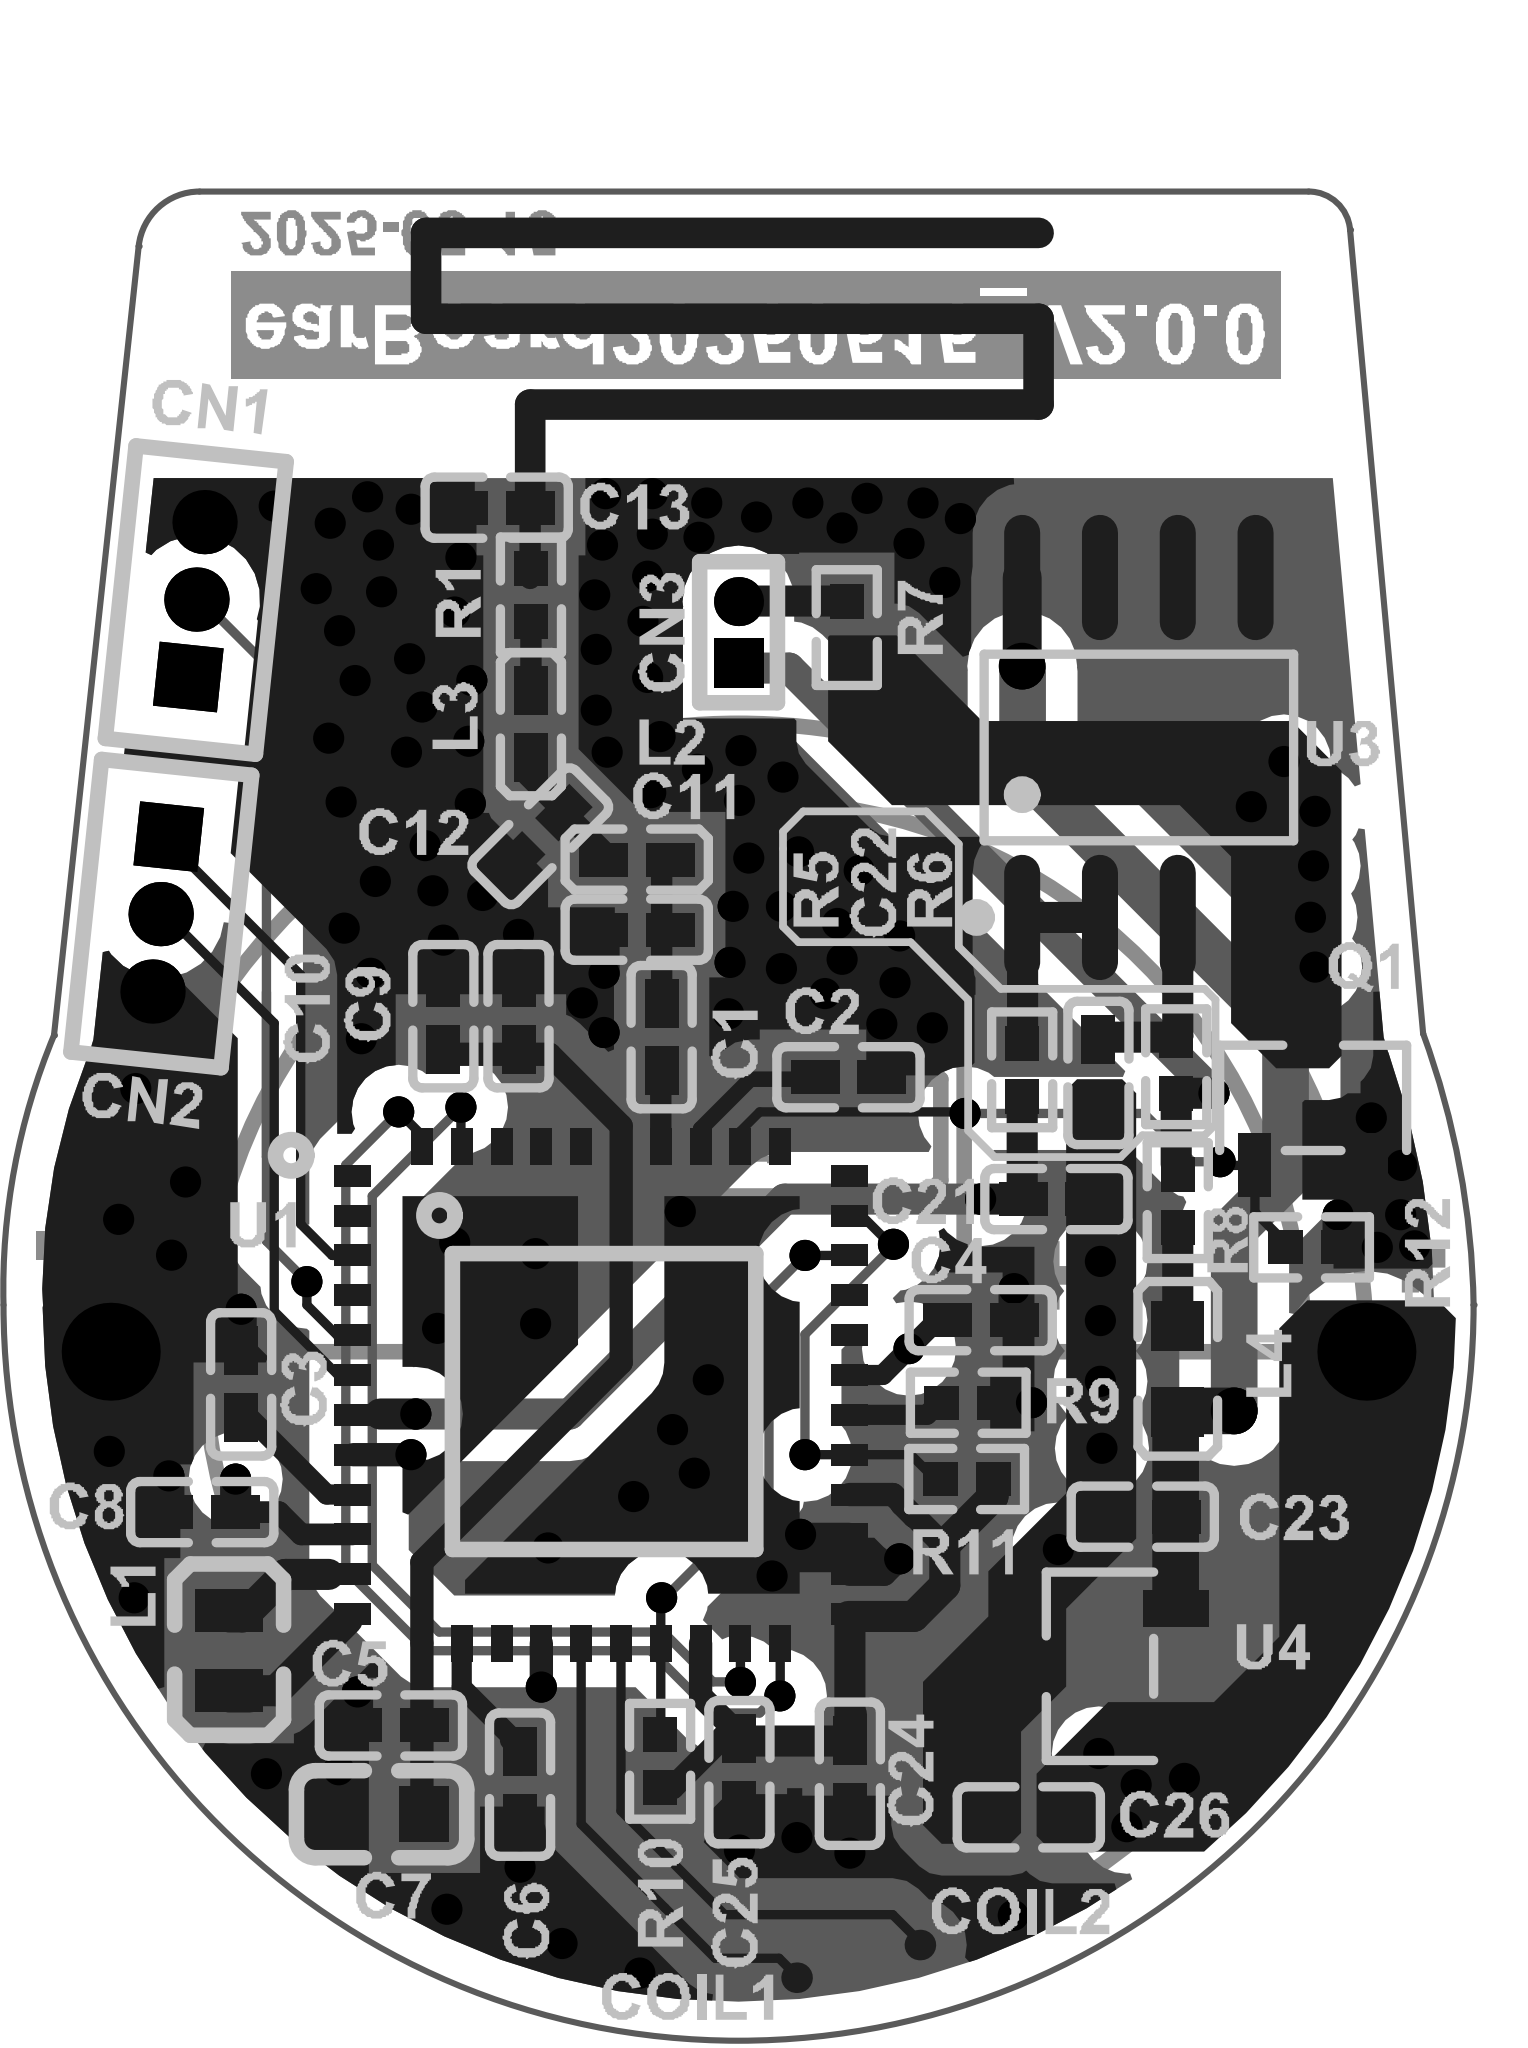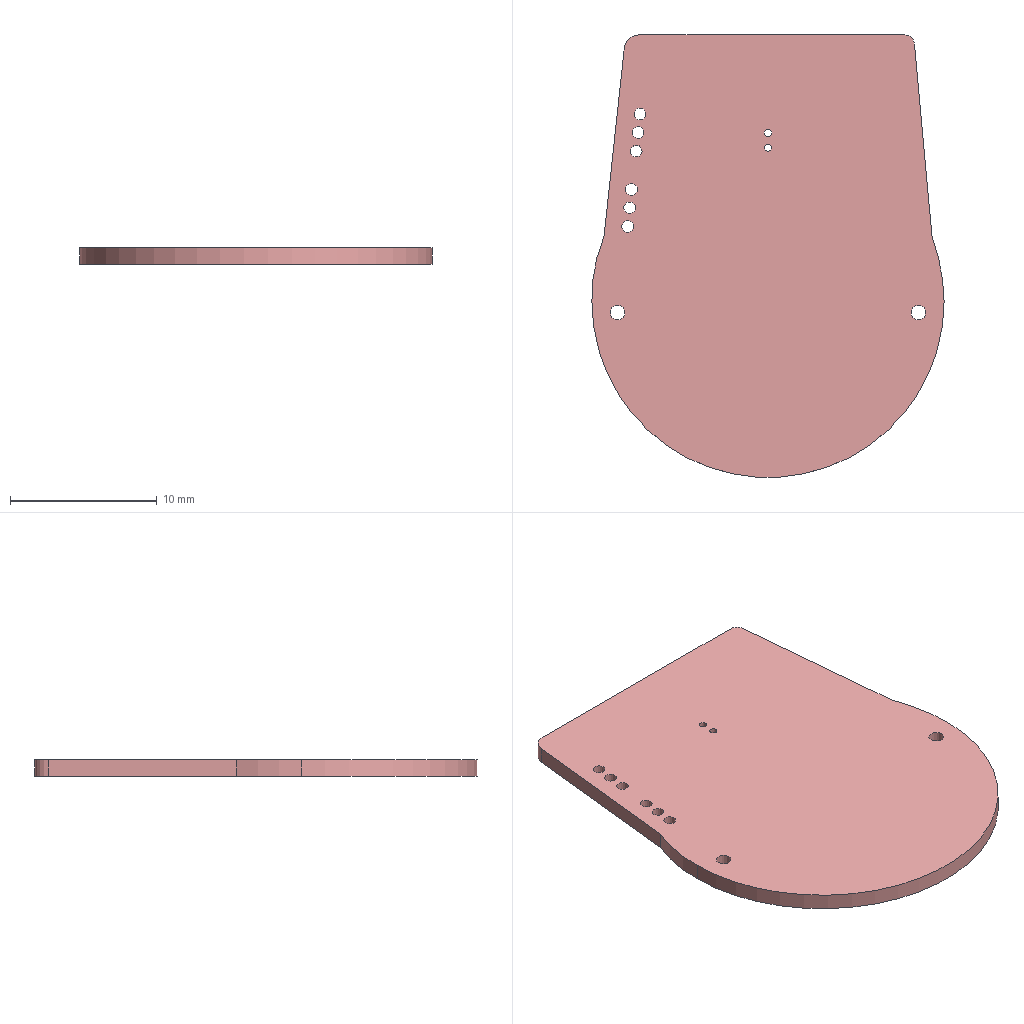Circuit board layout | Altium Designer | box 24 x 30.1 x 1.1 mm
Layer stack:
# Altium Designer layer stack of  (unit mm; dielectric type: 0 none, 1 core, 2 prepreg, 3 surface material)
index,name,kind,layer,copper_thickness_mm,dielectric_type,dielectric_thickness_mm,dielectric_material,dielectric_constant
0,Top Paste,other,,,,,,
1,Top Overlay,other,,,,,,
2,Top Solder,dielectric,,,3,0.0102,Solder Resist,3.5
3,Top Layer,copper,Top Layer,0.0356,,,,
4,Dielectric1,dielectric,,,1,0.32,FR-4,4.8
5,GND,copper,GND,0.0356,,,,
6,Dielectric2,dielectric,,,2,0.32,FR-4,4.8
7,POWER,copper,POWER,0.0356,,,,
8,Dielectric3,dielectric,,,1,0.32,FR-4,4.8
9,Bottom Layer,copper,Bottom Layer,0.0356,,,,
10,Bottom Solder,dielectric,,,3,0.0102,Solder Resist,3.5
11,Bottom Overlay,other,,,,,,
12,Bottom Paste,other,,,,,,
# drill layer pairs: low layer,high layer
drill_pair,Top Layer,Bottom Layer
Part placement:
Designator,Comment,Layer,Footprint,Center-X(mm),Center-Y(mm),Rotation
R1,,TopLayer,R0402,8.611,11.582,90
L2,2.4nH,TopLayer,L0402,10.338,7.264,180
C13,2pF,TopLayer,C0402,8.052,13.005,360
C11,2pF,TopLayer,C0402,10.338,6.121,360
L3,2.4nH,TopLayer,L0402,8.611,9.474,90
C12,2pF,TopLayer,C0402,8.763,7.645,45
C1,220pF,TopLayer,C0402,10.744,4.369,90
U2,Q&J CR2032 20-6*9,TopLayer,BAT-TH_CR2032,12,-0.7619,180
CN3,HX PZ1.0-1x2P ZZ,TopLayer,HDR-TH_2P-P1.00-V-M,12,10.973,90
R8,,TopLayer,R0402,19.17,1.702,270
R7,,TopLayer,R0402,13.767,11.049,90
R6,,TopLayer,R0402,19.145,3.886,90
U1,,TopLayer,KTYATR0101,9.755,-1.466,0
CN2,,TopLayer,HDR-TH_3P-P1.27-V-M-A,2.565,6.375,264
CN1,,TopLayer,HDR-TH_3P-P1.27-V-M-A,3.15,11.506,84
U4,REF3025AIDBZR,BottomLayer,SOT-23-3_L2.9-W1.6-P1.90-LS2.8-BR,17.9,-5.893,360
U3,MCP6022-I/SN,TopLayer,SOIC-8_L4.9-W3.9-P1.27-LS6.0-BL,18.535,9.094,360
R12,,TopLayer,R0402,21.355,0.9401,180
R11,,TopLayer,R0402,15.724,-2.838,360
R10,,TopLayer,R0402,10.719,-7.442,270
R9,,TopLayer,R0402,15.75,-1.593,180
R5,,TopLayer,R0402,16.63,3.836,90
Q1,BSS138,BottomLayer,SOT-23-3_L3.0-W1.7-P0.95-LS2.9-BR,21.38,3.378,270
L4,MPZ1608S101ATAH0,TopLayer,L0603,19.17,-1.041,270
L1,4.7uH,TopLayer,IND-SMD_L1.8-W1.2,3.683,-5.639,90
COIL2,,TopLayer,Test-Point-0.5mm,14.961,-10.439,0
COIL1,,TopLayer,Test-Point-0.5mm,12.947,-10.973,0
C26,470nF,TopLayer,C0402,16.739,-8.357,360
C25,0.1uF-c0402,TopLayer,C0402,12.014,-7.62,270
C24,0.1uF-c0402,TopLayer,C0402,13.818,-7.645,270
C23,100nF,TopLayer,C0402,18.599,-3.452,180
C22,100nF,TopLayer,C0402,17.875,3.785,90
C21,10pF,TopLayer,C0402,17.189,1.728,180
C10,0.1uF,TopLayer,C0402,7.181,4.71,270
C9,2.2uF,TopLayer,C0402,8.407,4.711,270
C8,1uF,TopLayer,C0402,3.245,-3.378,180
C7,0.1uF,TopLayer,C0603,6.172,-8.306,360
C6,1uF,TopLayer,C0402,8.433,-7.823,90
C5,1uF,TopLayer,C0402,6.325,-6.858,360
C4,1uF,TopLayer,C0402,15.953,-0.2473,180
C3,1uF,TopLayer,C0402,3.88,-1.295,270
C2,1uF,TopLayer,C0402,13.794,3.715,180
Pad and via stacks:
# Altium Designer via and pad stacks of  (unit mm). Each distinct definition once, with the count of objects using it.
# via: kind,start_layer,end_layer,hole_mm,diameter_mm,mode(0 simple;1 top-mid-bottom;2 full stack),diameter_per_layer,count,example_net
# pad: kind,layer,hole_mm,hole_type(0 round;1 square;2 slot),plating,top_size,top_shape(1 round;2 rect;3 octagon;9 rounded rect),mid_size,bottom_size,mode,footprint,size_per_layer,count,example
pad,Top Layer,0,0,plated,0.5657x0.54,2,0.5657x0.54,0.5657x0.54,0,R0402,,18,R1.2
pad,Top Layer,0,0,plated,0.7901x0.54,2,0.7901x0.54,0.7901x0.54,0,L0402,,4,L2.2
pad,Top Layer,0,0,plated,0.7901x0.54,2,0.7901x0.54,0.7901x0.54,0,C0402,,36,C13.2
pad,Top Layer,0,0,plated,0.6x0.35,2,0.6x0.35,0.6x0.35,0,KTYATR0101,,44,U1.34
pad,Top Layer,0,0,plated,0.588x2.045,1,0.588x2.045,0.588x2.045,0,SOIC-8_L4.9-W3.9-P1.27-LS6.0-BL,,8,U3.1
pad,Top Layer,0,0,plated,0.8x0.864,2,0.8x0.864,0.8x0.864,0,L0603,,2,L4.1
pad,Top Layer,0,0,plated,0.7x1.1,2,0.7x1.1,0.7x1.1,0,IND-SMD_L1.8-W1.2,,2,L1.1
pad,Top Layer,0,0,plated,0.5x0.5,1,0.5x0.5,0.5x0.5,0,Test-Point-0.5mm,,2,COIL2.1
pad,Top Layer,0,0,plated,0.8x0.9,2,0.8x0.9,0.8x0.9,0,C0603,,2,C7.2
pad,Top Layer,0,0,plated,1.038x0.532,2,1.038x0.532,1.038x0.532,0,SOT-23-3_L3.0-W1.7-P0.95-LS2.9-BR,,3,Q1.1
pad,Top Layer,0,0,plated,1.07x0.6,2,1.07x0.6,1.07x0.6,0,SOT-23-3_L2.9-W1.6-P1.90-LS2.8-BR,,3,U4.1
pad,Multi-Layer,1,0,plated,1.6x1.6,1,1.6x1.6,1.6x1.6,0,BAT-TH_CR2032,,2,U2.1
pad,Multi-Layer,0.5,0,plated,0.8x0.8,1,0.8x0.8,0.8x0.8,0,HDR-TH_2P-P1.00-V-M,,1,CN3.2
pad,Multi-Layer,0.5,0,plated,0.8x0.8,2,0.8x0.8,0.8x0.8,0,HDR-TH_2P-P1.00-V-M,,1,CN3.1
pad,Multi-Layer,0.8,0,plated,1.05x1.05,2,1.05x1.05,1.05x1.05,0,HDR-TH_3P-P1.27-V-M-A,,2,CN2.1
pad,Multi-Layer,0.8,0,plated,1.05x1.05,1,1.05x1.05,1.05x1.05,0,HDR-TH_3P-P1.27-V-M-A,,4,CN2.2
via,Top Layer,Bottom Layer,0.3048,0.508,0,,146,GND
via,Top Layer,Bottom Layer,0.381,0.762,0,,2,NetC23_1
Copper pours:
name,layer,net,type(0 solid;1 hatched;2 none)
Bottom Layer-No Net,Top Layer,NetC21_1,0
Bottom Layer-No Net,Top Layer,NetC21_1,0
Bottom Layer-No Net,Top Layer,TL_VDD3,0
Bottom Layer-No Net,Top Layer,GND,0
Bottom Layer-No Net,Bottom Layer,GND,0
Design rules, without the lines most boards share:
# Altium Designer design rules of  (exported by Altium Designer, unit mm)
# columns: name | kind | enabled | priority | scope1 | scope2 | descriptor | typed fields (field=value)
Clearance | 0 | enabled | 2 | All | All | Clearance Constraint (Gap=6mil) (All),(All) | gap=0.1524
PlaneConnect | 6 | enabled | 1 | All | All | Power Plane Connect Rule(Direct Connect )(Expansion=20mil) (Conductor Width=10mil) (Air Gap=10mil) (Entries=4) (All) | relief_conductor_width=0.254 relief_entries=4 relief_expansion=0.508
PlaneClearance | 12 | enabled | 1 | All | All | Power Plane Clearance (Clearance =6mil) (All) | clearance=0.1524
PolygonConnect | 20 | enabled | 1 | All | All | Polygon Connect Rule(Direct Connect )(Conductor Width=10mil) (Relief Angle=90 Angle) (Entries=4) (Air Gap Width=10mil) (All),(All) | connect_style(0=relief,1=direct,2=none)=1 relief_conductor_width=0.254 relief_entries=4
Width | 2 | enabled | 1 | All | All | Width Constraint (Min=6mil) (Max=40mil) (Preferred=10mil) (All) |
RoutingVias | 11 | enabled | 1 | All | All | Routing Via (MinHoleWidth=12mil) (MaxHoleWidth=12mil) (PreferredHoleWidth=12mil) (MinWidth=20mil) (MaxWidth=20mil) (PreferedWidth=20mil) (All) | via_min_hole=0.3048 via_max_hole=0.3048 via_preferred_diameter=0.508 via_preferred_hole=0.3048
SolderMaskExpansion | 13 | enabled | 1 | All | All | Solder Mask Expansion (Expansion =4mil) (All) | expansion=0.1016
HoleSize | 42 | enabled | 1 | All | All | Hole Size Constraint (Min=1mil) (Max=500mil) (All) |
DiffPairsRouting | 51 | enabled | 1 | All | All | Differential Pairs Uncoupled Length using the Gap Constraints (Min=6mil) (Max=6mil) (Prefered=6mil)  and Width Constraints (Min=15mil) (Max=15mil) (Prefered=15mil) (All) |
HoleToHoleClearance | 52 | enabled | 1 | All | All | Hole To Hole Clearance (Gap=0mil) (All),(All) | gap=0
MinimumSolderMaskSliver | 53 | enabled | 1 | All | All | Minimum Solder Mask Sliver (Gap=0mil) (All),(All) |
SilkscreenOverComponentPads | 54 | enabled | 1 | IsPad | All | Silk To Solder Mask (Clearance=0mil) (IsPad),(All) |
SilkToSilkClearance | 55 | enabled | 1 | All | All | Silk to Silk (Clearance=0mil) (All),(All) |
Clearance_1 | 0 | enabled | 1 | inpolygon | All | Clearance Constraint (Gap=6mil) (inpolygon),(All) | gap=0.1524